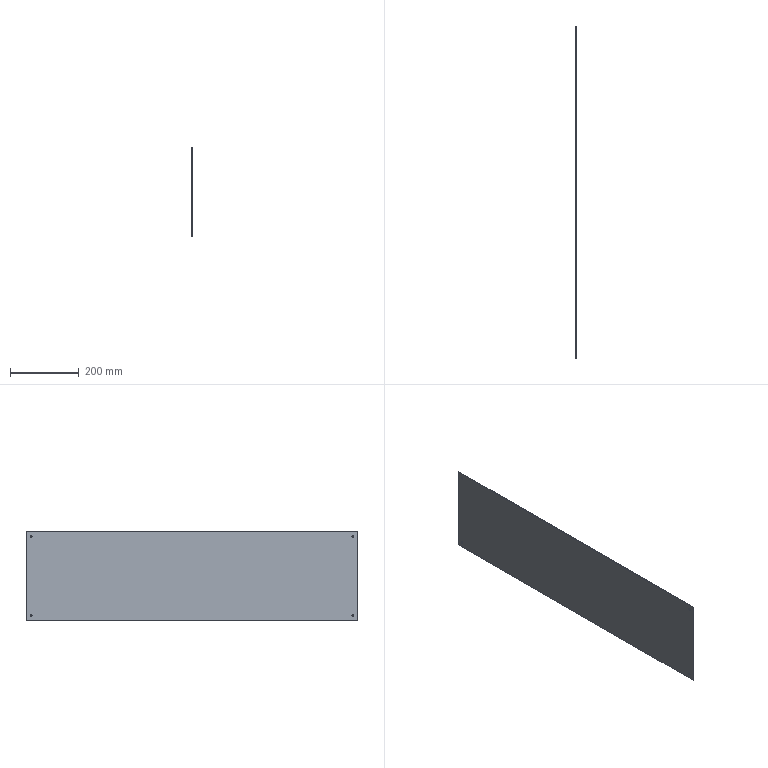Part | STEP file | PA-7-65(cover plate) | 1 solid | 14 faces | box 2 x 968 x 260 mm | volume 503203 mm3 | cylinder 8 | plane 6 | commonest cylinder face diameters 5 x8
STEP:
#1=CARTESIAN_POINT('',(0.,0.,0.));
#2=DIRECTION('',(0.,0.,1.));
#3=DIRECTION('',(1.,0.,0.));
#4=AXIS2_PLACEMENT_3D('',#1,#2,#3);
#5=CARTESIAN_POINT('',(-2.,469.,112.5));
#6=VERTEX_POINT('',#5);
#7=CARTESIAN_POINT('',(0.,469.,112.5));
#8=VERTEX_POINT('',#7);
#9=CARTESIAN_POINT('',(0.,469.,112.5));
#10=DIRECTION('',(1.,0.,0.));
#11=VECTOR('',#10,1.);
#12=LINE('',#9,#11);
#13=CARTESIAN_POINT('',(0.,469.,115.));
#14=DIRECTION('',(1.,0.,0.));
#15=DIRECTION('',(0.,0.,-1.));
#16=AXIS2_PLACEMENT_3D('',#13,#14,#15);
#17=CYLINDRICAL_SURFACE('',#16,2.5);
#18=CARTESIAN_POINT('',(6.283,0.));
#19=DIRECTION('',(0.,1.));
#20=VECTOR('',#19,1.);
#21=LINE('',#18,#20);
#22=(GEOMETRIC_REPRESENTATION_CONTEXT(2)PARAMETRIC_REPRESENTATION_CONTEXT()REPRESENTATION_CONTEXT('',''));
#23=DEFINITIONAL_REPRESENTATION('',(#21),#22);
#24=PCURVE('',#17,#23);
#25=CARTESIAN_POINT('',(0.,469.,115.));
#26=DIRECTION('',(1.,0.,0.));
#27=DIRECTION('',(0.,0.,-1.));
#28=AXIS2_PLACEMENT_3D('',#25,#26,#27);
#29=CYLINDRICAL_SURFACE('',#28,2.5);
#30=CARTESIAN_POINT('',(0.,0.));
#31=DIRECTION('',(0.,1.));
#32=VECTOR('',#31,1.);
#33=LINE('',#30,#32);
#34=(GEOMETRIC_REPRESENTATION_CONTEXT(2)PARAMETRIC_REPRESENTATION_CONTEXT()REPRESENTATION_CONTEXT('',''));
#35=DEFINITIONAL_REPRESENTATION('',(#33),#34);
#36=PCURVE('',#29,#35);
#37=SURFACE_CURVE('',#12,(#24,#36),.PCURVE_S1.);
#38=EDGE_CURVE('',#6,#8,#37,.T.);
#39=ORIENTED_EDGE('',*,*,#38,.T.);
#40=CARTESIAN_POINT('',(0.,469.,117.5));
#41=VERTEX_POINT('',#40);
#42=CARTESIAN_POINT('',(0.,469.,115.));
#43=DIRECTION('',(1.,0.,0.));
#44=DIRECTION('',(0.,0.,-1.));
#45=AXIS2_PLACEMENT_3D('',#42,#43,#44);
#46=CIRCLE('',#45,2.5);
#47=CARTESIAN_POINT('',(0.,0.));
#48=DIRECTION('',(1.,0.));
#49=VECTOR('',#48,1.);
#50=LINE('',#47,#49);
#51=(GEOMETRIC_REPRESENTATION_CONTEXT(2)PARAMETRIC_REPRESENTATION_CONTEXT()REPRESENTATION_CONTEXT('',''));
#52=DEFINITIONAL_REPRESENTATION('',(#50),#51);
#53=PCURVE('',#17,#52);
#54=CARTESIAN_POINT('',(0.,0.,0.));
#55=DIRECTION('',(1.,0.,0.));
#56=DIRECTION('',(0.,0.,-1.));
#57=AXIS2_PLACEMENT_3D('',#54,#55,#56);
#58=PLANE('',#57);
#59=CARTESIAN_POINT('',(-115.,469.));
#60=DIRECTION('',(1.,0.));
#61=AXIS2_PLACEMENT_2D('',#59,#60);
#62=CIRCLE('',#61,2.5);
#63=(GEOMETRIC_REPRESENTATION_CONTEXT(2)PARAMETRIC_REPRESENTATION_CONTEXT()REPRESENTATION_CONTEXT('',''));
#64=DEFINITIONAL_REPRESENTATION('',(#62),#63);
#65=PCURVE('',#58,#64);
#66=SURFACE_CURVE('',#46,(#53,#65),.PCURVE_S1.);
#67=EDGE_CURVE('',#41,#8,#66,.T.);
#68=ORIENTED_EDGE('',*,*,#67,.F.);
#69=CARTESIAN_POINT('',(-2.,469.,117.5));
#70=VERTEX_POINT('',#69);
#71=CARTESIAN_POINT('',(0.,469.,117.5));
#72=DIRECTION('',(1.,0.,0.));
#73=VECTOR('',#72,1.);
#74=LINE('',#71,#73);
#75=CARTESIAN_POINT('',(3.142,0.));
#76=DIRECTION('',(0.,1.));
#77=VECTOR('',#76,1.);
#78=LINE('',#75,#77);
#79=(GEOMETRIC_REPRESENTATION_CONTEXT(2)PARAMETRIC_REPRESENTATION_CONTEXT()REPRESENTATION_CONTEXT('',''));
#80=DEFINITIONAL_REPRESENTATION('',(#78),#79);
#81=PCURVE('',#17,#80);
#82=CARTESIAN_POINT('',(3.142,0.));
#83=DIRECTION('',(0.,1.));
#84=VECTOR('',#83,1.);
#85=LINE('',#82,#84);
#86=(GEOMETRIC_REPRESENTATION_CONTEXT(2)PARAMETRIC_REPRESENTATION_CONTEXT()REPRESENTATION_CONTEXT('',''));
#87=DEFINITIONAL_REPRESENTATION('',(#85),#86);
#88=PCURVE('',#29,#87);
#89=SURFACE_CURVE('',#74,(#81,#88),.PCURVE_S1.);
#90=EDGE_CURVE('',#70,#41,#89,.T.);
#91=ORIENTED_EDGE('',*,*,#90,.F.);
#92=CARTESIAN_POINT('',(-2.,469.,115.));
#93=DIRECTION('',(1.,0.,0.));
#94=DIRECTION('',(0.,0.,-1.));
#95=AXIS2_PLACEMENT_3D('',#92,#93,#94);
#96=CIRCLE('',#95,2.5);
#97=CARTESIAN_POINT('',(0.,-2.));
#98=DIRECTION('',(1.,0.));
#99=VECTOR('',#98,1.);
#100=LINE('',#97,#99);
#101=(GEOMETRIC_REPRESENTATION_CONTEXT(2)PARAMETRIC_REPRESENTATION_CONTEXT()REPRESENTATION_CONTEXT('',''));
#102=DEFINITIONAL_REPRESENTATION('',(#100),#101);
#103=PCURVE('',#17,#102);
#104=CARTESIAN_POINT('',(-2.,0.,0.));
#105=DIRECTION('',(1.,0.,0.));
#106=DIRECTION('',(0.,0.,-1.));
#107=AXIS2_PLACEMENT_3D('',#104,#105,#106);
#108=PLANE('',#107);
#109=CARTESIAN_POINT('',(-115.,469.));
#110=DIRECTION('',(1.,0.));
#111=AXIS2_PLACEMENT_2D('',#109,#110);
#112=CIRCLE('',#111,2.5);
#113=(GEOMETRIC_REPRESENTATION_CONTEXT(2)PARAMETRIC_REPRESENTATION_CONTEXT()REPRESENTATION_CONTEXT('',''));
#114=DEFINITIONAL_REPRESENTATION('',(#112),#113);
#115=PCURVE('',#108,#114);
#116=SURFACE_CURVE('',#96,(#103,#115),.PCURVE_S1.);
#117=EDGE_CURVE('',#70,#6,#116,.T.);
#118=ORIENTED_EDGE('',*,*,#117,.T.);
#119=EDGE_LOOP('',(#39,#68,#91,#118));
#120=FACE_BOUND('',#119,.F.);
#121=ADVANCED_FACE('',(#120),#17,.F.);
#122=CARTESIAN_POINT('',(-2.,-469.,112.5));
#123=VERTEX_POINT('',#122);
#124=CARTESIAN_POINT('',(0.,-469.,112.5));
#125=VERTEX_POINT('',#124);
#126=CARTESIAN_POINT('',(0.,-469.,112.5));
#127=DIRECTION('',(1.,0.,0.));
#128=VECTOR('',#127,1.);
#129=LINE('',#126,#128);
#130=CARTESIAN_POINT('',(0.,-469.,115.));
#131=DIRECTION('',(1.,0.,0.));
#132=DIRECTION('',(0.,0.,-1.));
#133=AXIS2_PLACEMENT_3D('',#130,#131,#132);
#134=CYLINDRICAL_SURFACE('',#133,2.5);
#135=CARTESIAN_POINT('',(6.283,0.));
#136=DIRECTION('',(0.,1.));
#137=VECTOR('',#136,1.);
#138=LINE('',#135,#137);
#139=(GEOMETRIC_REPRESENTATION_CONTEXT(2)PARAMETRIC_REPRESENTATION_CONTEXT()REPRESENTATION_CONTEXT('',''));
#140=DEFINITIONAL_REPRESENTATION('',(#138),#139);
#141=PCURVE('',#134,#140);
#142=CARTESIAN_POINT('',(0.,-469.,115.));
#143=DIRECTION('',(1.,0.,0.));
#144=DIRECTION('',(0.,0.,-1.));
#145=AXIS2_PLACEMENT_3D('',#142,#143,#144);
#146=CYLINDRICAL_SURFACE('',#145,2.5);
#147=CARTESIAN_POINT('',(0.,0.));
#148=DIRECTION('',(0.,1.));
#149=VECTOR('',#148,1.);
#150=LINE('',#147,#149);
#151=(GEOMETRIC_REPRESENTATION_CONTEXT(2)PARAMETRIC_REPRESENTATION_CONTEXT()REPRESENTATION_CONTEXT('',''));
#152=DEFINITIONAL_REPRESENTATION('',(#150),#151);
#153=PCURVE('',#146,#152);
#154=SURFACE_CURVE('',#129,(#141,#153),.PCURVE_S1.);
#155=EDGE_CURVE('',#123,#125,#154,.T.);
#156=ORIENTED_EDGE('',*,*,#155,.T.);
#157=CARTESIAN_POINT('',(0.,-469.,117.5));
#158=VERTEX_POINT('',#157);
#159=CARTESIAN_POINT('',(0.,-469.,115.));
#160=DIRECTION('',(1.,0.,0.));
#161=DIRECTION('',(0.,0.,-1.));
#162=AXIS2_PLACEMENT_3D('',#159,#160,#161);
#163=CIRCLE('',#162,2.5);
#164=CARTESIAN_POINT('',(0.,0.));
#165=DIRECTION('',(1.,0.));
#166=VECTOR('',#165,1.);
#167=LINE('',#164,#166);
#168=(GEOMETRIC_REPRESENTATION_CONTEXT(2)PARAMETRIC_REPRESENTATION_CONTEXT()REPRESENTATION_CONTEXT('',''));
#169=DEFINITIONAL_REPRESENTATION('',(#167),#168);
#170=PCURVE('',#134,#169);
#171=CARTESIAN_POINT('',(-115.,-469.));
#172=DIRECTION('',(1.,0.));
#173=AXIS2_PLACEMENT_2D('',#171,#172);
#174=CIRCLE('',#173,2.5);
#175=(GEOMETRIC_REPRESENTATION_CONTEXT(2)PARAMETRIC_REPRESENTATION_CONTEXT()REPRESENTATION_CONTEXT('',''));
#176=DEFINITIONAL_REPRESENTATION('',(#174),#175);
#177=PCURVE('',#58,#176);
#178=SURFACE_CURVE('',#163,(#170,#177),.PCURVE_S1.);
#179=EDGE_CURVE('',#158,#125,#178,.T.);
#180=ORIENTED_EDGE('',*,*,#179,.F.);
#181=CARTESIAN_POINT('',(-2.,-469.,117.5));
#182=VERTEX_POINT('',#181);
#183=CARTESIAN_POINT('',(0.,-469.,117.5));
#184=DIRECTION('',(1.,0.,0.));
#185=VECTOR('',#184,1.);
#186=LINE('',#183,#185);
#187=CARTESIAN_POINT('',(3.142,0.));
#188=DIRECTION('',(0.,1.));
#189=VECTOR('',#188,1.);
#190=LINE('',#187,#189);
#191=(GEOMETRIC_REPRESENTATION_CONTEXT(2)PARAMETRIC_REPRESENTATION_CONTEXT()REPRESENTATION_CONTEXT('',''));
#192=DEFINITIONAL_REPRESENTATION('',(#190),#191);
#193=PCURVE('',#134,#192);
#194=CARTESIAN_POINT('',(3.142,0.));
#195=DIRECTION('',(0.,1.));
#196=VECTOR('',#195,1.);
#197=LINE('',#194,#196);
#198=(GEOMETRIC_REPRESENTATION_CONTEXT(2)PARAMETRIC_REPRESENTATION_CONTEXT()REPRESENTATION_CONTEXT('',''));
#199=DEFINITIONAL_REPRESENTATION('',(#197),#198);
#200=PCURVE('',#146,#199);
#201=SURFACE_CURVE('',#186,(#193,#200),.PCURVE_S1.);
#202=EDGE_CURVE('',#182,#158,#201,.T.);
#203=ORIENTED_EDGE('',*,*,#202,.F.);
#204=CARTESIAN_POINT('',(-2.,-469.,115.));
#205=DIRECTION('',(1.,0.,0.));
#206=DIRECTION('',(0.,0.,-1.));
#207=AXIS2_PLACEMENT_3D('',#204,#205,#206);
#208=CIRCLE('',#207,2.5);
#209=CARTESIAN_POINT('',(0.,-2.));
#210=DIRECTION('',(1.,0.));
#211=VECTOR('',#210,1.);
#212=LINE('',#209,#211);
#213=(GEOMETRIC_REPRESENTATION_CONTEXT(2)PARAMETRIC_REPRESENTATION_CONTEXT()REPRESENTATION_CONTEXT('',''));
#214=DEFINITIONAL_REPRESENTATION('',(#212),#213);
#215=PCURVE('',#134,#214);
#216=CARTESIAN_POINT('',(-115.,-469.));
#217=DIRECTION('',(1.,0.));
#218=AXIS2_PLACEMENT_2D('',#216,#217);
#219=CIRCLE('',#218,2.5);
#220=(GEOMETRIC_REPRESENTATION_CONTEXT(2)PARAMETRIC_REPRESENTATION_CONTEXT()REPRESENTATION_CONTEXT('',''));
#221=DEFINITIONAL_REPRESENTATION('',(#219),#220);
#222=PCURVE('',#108,#221);
#223=SURFACE_CURVE('',#208,(#215,#222),.PCURVE_S1.);
#224=EDGE_CURVE('',#182,#123,#223,.T.);
#225=ORIENTED_EDGE('',*,*,#224,.T.);
#226=EDGE_LOOP('',(#156,#180,#203,#225));
#227=FACE_BOUND('',#226,.F.);
#228=ADVANCED_FACE('',(#227),#134,.F.);
#229=CARTESIAN_POINT('',(-2.,-469.,-117.5));
#230=VERTEX_POINT('',#229);
#231=CARTESIAN_POINT('',(0.,-469.,-117.5));
#232=VERTEX_POINT('',#231);
#233=CARTESIAN_POINT('',(0.,-469.,-117.5));
#234=DIRECTION('',(1.,0.,0.));
#235=VECTOR('',#234,1.);
#236=LINE('',#233,#235);
#237=CARTESIAN_POINT('',(0.,-469.,-115.));
#238=DIRECTION('',(1.,0.,0.));
#239=DIRECTION('',(0.,0.,-1.));
#240=AXIS2_PLACEMENT_3D('',#237,#238,#239);
#241=CYLINDRICAL_SURFACE('',#240,2.5);
#242=CARTESIAN_POINT('',(6.283,0.));
#243=DIRECTION('',(0.,1.));
#244=VECTOR('',#243,1.);
#245=LINE('',#242,#244);
#246=(GEOMETRIC_REPRESENTATION_CONTEXT(2)PARAMETRIC_REPRESENTATION_CONTEXT()REPRESENTATION_CONTEXT('',''));
#247=DEFINITIONAL_REPRESENTATION('',(#245),#246);
#248=PCURVE('',#241,#247);
#249=CARTESIAN_POINT('',(0.,-469.,-115.));
#250=DIRECTION('',(1.,0.,0.));
#251=DIRECTION('',(0.,0.,-1.));
#252=AXIS2_PLACEMENT_3D('',#249,#250,#251);
#253=CYLINDRICAL_SURFACE('',#252,2.5);
#254=CARTESIAN_POINT('',(0.,0.));
#255=DIRECTION('',(0.,1.));
#256=VECTOR('',#255,1.);
#257=LINE('',#254,#256);
#258=(GEOMETRIC_REPRESENTATION_CONTEXT(2)PARAMETRIC_REPRESENTATION_CONTEXT()REPRESENTATION_CONTEXT('',''));
#259=DEFINITIONAL_REPRESENTATION('',(#257),#258);
#260=PCURVE('',#253,#259);
#261=SURFACE_CURVE('',#236,(#248,#260),.PCURVE_S1.);
#262=EDGE_CURVE('',#230,#232,#261,.T.);
#263=ORIENTED_EDGE('',*,*,#262,.T.);
#264=CARTESIAN_POINT('',(0.,-469.,-112.5));
#265=VERTEX_POINT('',#264);
#266=CARTESIAN_POINT('',(0.,-469.,-115.));
#267=DIRECTION('',(1.,0.,0.));
#268=DIRECTION('',(0.,0.,-1.));
#269=AXIS2_PLACEMENT_3D('',#266,#267,#268);
#270=CIRCLE('',#269,2.5);
#271=CARTESIAN_POINT('',(0.,0.));
#272=DIRECTION('',(1.,0.));
#273=VECTOR('',#272,1.);
#274=LINE('',#271,#273);
#275=(GEOMETRIC_REPRESENTATION_CONTEXT(2)PARAMETRIC_REPRESENTATION_CONTEXT()REPRESENTATION_CONTEXT('',''));
#276=DEFINITIONAL_REPRESENTATION('',(#274),#275);
#277=PCURVE('',#241,#276);
#278=CARTESIAN_POINT('',(115.,-469.));
#279=DIRECTION('',(1.,0.));
#280=AXIS2_PLACEMENT_2D('',#278,#279);
#281=CIRCLE('',#280,2.5);
#282=(GEOMETRIC_REPRESENTATION_CONTEXT(2)PARAMETRIC_REPRESENTATION_CONTEXT()REPRESENTATION_CONTEXT('',''));
#283=DEFINITIONAL_REPRESENTATION('',(#281),#282);
#284=PCURVE('',#58,#283);
#285=SURFACE_CURVE('',#270,(#277,#284),.PCURVE_S1.);
#286=EDGE_CURVE('',#265,#232,#285,.T.);
#287=ORIENTED_EDGE('',*,*,#286,.F.);
#288=CARTESIAN_POINT('',(-2.,-469.,-112.5));
#289=VERTEX_POINT('',#288);
#290=CARTESIAN_POINT('',(0.,-469.,-112.5));
#291=DIRECTION('',(1.,0.,0.));
#292=VECTOR('',#291,1.);
#293=LINE('',#290,#292);
#294=CARTESIAN_POINT('',(3.142,0.));
#295=DIRECTION('',(0.,1.));
#296=VECTOR('',#295,1.);
#297=LINE('',#294,#296);
#298=(GEOMETRIC_REPRESENTATION_CONTEXT(2)PARAMETRIC_REPRESENTATION_CONTEXT()REPRESENTATION_CONTEXT('',''));
#299=DEFINITIONAL_REPRESENTATION('',(#297),#298);
#300=PCURVE('',#241,#299);
#301=CARTESIAN_POINT('',(3.142,0.));
#302=DIRECTION('',(0.,1.));
#303=VECTOR('',#302,1.);
#304=LINE('',#301,#303);
#305=(GEOMETRIC_REPRESENTATION_CONTEXT(2)PARAMETRIC_REPRESENTATION_CONTEXT()REPRESENTATION_CONTEXT('',''));
#306=DEFINITIONAL_REPRESENTATION('',(#304),#305);
#307=PCURVE('',#253,#306);
#308=SURFACE_CURVE('',#293,(#300,#307),.PCURVE_S1.);
#309=EDGE_CURVE('',#289,#265,#308,.T.);
#310=ORIENTED_EDGE('',*,*,#309,.F.);
#311=CARTESIAN_POINT('',(-2.,-469.,-115.));
#312=DIRECTION('',(1.,0.,0.));
#313=DIRECTION('',(0.,0.,-1.));
#314=AXIS2_PLACEMENT_3D('',#311,#312,#313);
#315=CIRCLE('',#314,2.5);
#316=CARTESIAN_POINT('',(0.,-2.));
#317=DIRECTION('',(1.,0.));
#318=VECTOR('',#317,1.);
#319=LINE('',#316,#318);
#320=(GEOMETRIC_REPRESENTATION_CONTEXT(2)PARAMETRIC_REPRESENTATION_CONTEXT()REPRESENTATION_CONTEXT('',''));
#321=DEFINITIONAL_REPRESENTATION('',(#319),#320);
#322=PCURVE('',#241,#321);
#323=CARTESIAN_POINT('',(115.,-469.));
#324=DIRECTION('',(1.,0.));
#325=AXIS2_PLACEMENT_2D('',#323,#324);
#326=CIRCLE('',#325,2.5);
#327=(GEOMETRIC_REPRESENTATION_CONTEXT(2)PARAMETRIC_REPRESENTATION_CONTEXT()REPRESENTATION_CONTEXT('',''));
#328=DEFINITIONAL_REPRESENTATION('',(#326),#327);
#329=PCURVE('',#108,#328);
#330=SURFACE_CURVE('',#315,(#322,#329),.PCURVE_S1.);
#331=EDGE_CURVE('',#289,#230,#330,.T.);
#332=ORIENTED_EDGE('',*,*,#331,.T.);
#333=EDGE_LOOP('',(#263,#287,#310,#332));
#334=FACE_BOUND('',#333,.F.);
#335=ADVANCED_FACE('',(#334),#241,.F.);
#336=CARTESIAN_POINT('',(-2.,469.,-117.5));
#337=VERTEX_POINT('',#336);
#338=CARTESIAN_POINT('',(0.,469.,-117.5));
#339=VERTEX_POINT('',#338);
#340=CARTESIAN_POINT('',(0.,469.,-117.5));
#341=DIRECTION('',(1.,0.,0.));
#342=VECTOR('',#341,1.);
#343=LINE('',#340,#342);
#344=CARTESIAN_POINT('',(0.,469.,-115.));
#345=DIRECTION('',(1.,0.,0.));
#346=DIRECTION('',(0.,0.,-1.));
#347=AXIS2_PLACEMENT_3D('',#344,#345,#346);
#348=CYLINDRICAL_SURFACE('',#347,2.5);
#349=CARTESIAN_POINT('',(6.283,0.));
#350=DIRECTION('',(0.,1.));
#351=VECTOR('',#350,1.);
#352=LINE('',#349,#351);
#353=(GEOMETRIC_REPRESENTATION_CONTEXT(2)PARAMETRIC_REPRESENTATION_CONTEXT()REPRESENTATION_CONTEXT('',''));
#354=DEFINITIONAL_REPRESENTATION('',(#352),#353);
#355=PCURVE('',#348,#354);
#356=CARTESIAN_POINT('',(0.,469.,-115.));
#357=DIRECTION('',(1.,0.,0.));
#358=DIRECTION('',(0.,0.,-1.));
#359=AXIS2_PLACEMENT_3D('',#356,#357,#358);
#360=CYLINDRICAL_SURFACE('',#359,2.5);
#361=CARTESIAN_POINT('',(0.,0.));
#362=DIRECTION('',(0.,1.));
#363=VECTOR('',#362,1.);
#364=LINE('',#361,#363);
#365=(GEOMETRIC_REPRESENTATION_CONTEXT(2)PARAMETRIC_REPRESENTATION_CONTEXT()REPRESENTATION_CONTEXT('',''));
#366=DEFINITIONAL_REPRESENTATION('',(#364),#365);
#367=PCURVE('',#360,#366);
#368=SURFACE_CURVE('',#343,(#355,#367),.PCURVE_S1.);
#369=EDGE_CURVE('',#337,#339,#368,.T.);
#370=ORIENTED_EDGE('',*,*,#369,.T.);
#371=CARTESIAN_POINT('',(0.,469.,-112.5));
#372=VERTEX_POINT('',#371);
#373=CARTESIAN_POINT('',(0.,469.,-115.));
#374=DIRECTION('',(1.,0.,0.));
#375=DIRECTION('',(0.,0.,-1.));
#376=AXIS2_PLACEMENT_3D('',#373,#374,#375);
#377=CIRCLE('',#376,2.5);
#378=CARTESIAN_POINT('',(0.,0.));
#379=DIRECTION('',(1.,0.));
#380=VECTOR('',#379,1.);
#381=LINE('',#378,#380);
#382=(GEOMETRIC_REPRESENTATION_CONTEXT(2)PARAMETRIC_REPRESENTATION_CONTEXT()REPRESENTATION_CONTEXT('',''));
#383=DEFINITIONAL_REPRESENTATION('',(#381),#382);
#384=PCURVE('',#348,#383);
#385=CARTESIAN_POINT('',(115.,469.));
#386=DIRECTION('',(1.,0.));
#387=AXIS2_PLACEMENT_2D('',#385,#386);
#388=CIRCLE('',#387,2.5);
#389=(GEOMETRIC_REPRESENTATION_CONTEXT(2)PARAMETRIC_REPRESENTATION_CONTEXT()REPRESENTATION_CONTEXT('',''));
#390=DEFINITIONAL_REPRESENTATION('',(#388),#389);
#391=PCURVE('',#58,#390);
#392=SURFACE_CURVE('',#377,(#384,#391),.PCURVE_S1.);
#393=EDGE_CURVE('',#372,#339,#392,.T.);
#394=ORIENTED_EDGE('',*,*,#393,.F.);
#395=CARTESIAN_POINT('',(-2.,469.,-112.5));
#396=VERTEX_POINT('',#395);
#397=CARTESIAN_POINT('',(0.,469.,-112.5));
#398=DIRECTION('',(1.,0.,0.));
#399=VECTOR('',#398,1.);
#400=LINE('',#397,#399);
#401=CARTESIAN_POINT('',(3.142,0.));
#402=DIRECTION('',(0.,1.));
#403=VECTOR('',#402,1.);
#404=LINE('',#401,#403);
#405=(GEOMETRIC_REPRESENTATION_CONTEXT(2)PARAMETRIC_REPRESENTATION_CONTEXT()REPRESENTATION_CONTEXT('',''));
#406=DEFINITIONAL_REPRESENTATION('',(#404),#405);
#407=PCURVE('',#348,#406);
#408=CARTESIAN_POINT('',(3.142,0.));
#409=DIRECTION('',(0.,1.));
#410=VECTOR('',#409,1.);
#411=LINE('',#408,#410);
#412=(GEOMETRIC_REPRESENTATION_CONTEXT(2)PARAMETRIC_REPRESENTATION_CONTEXT()REPRESENTATION_CONTEXT('',''));
#413=DEFINITIONAL_REPRESENTATION('',(#411),#412);
#414=PCURVE('',#360,#413);
#415=SURFACE_CURVE('',#400,(#407,#414),.PCURVE_S1.);
#416=EDGE_CURVE('',#396,#372,#415,.T.);
#417=ORIENTED_EDGE('',*,*,#416,.F.);
#418=CARTESIAN_POINT('',(-2.,469.,-115.));
#419=DIRECTION('',(1.,0.,0.));
#420=DIRECTION('',(0.,0.,-1.));
#421=AXIS2_PLACEMENT_3D('',#418,#419,#420);
#422=CIRCLE('',#421,2.5);
#423=CARTESIAN_POINT('',(0.,-2.));
#424=DIRECTION('',(1.,0.));
#425=VECTOR('',#424,1.);
#426=LINE('',#423,#425);
#427=(GEOMETRIC_REPRESENTATION_CONTEXT(2)PARAMETRIC_REPRESENTATION_CONTEXT()REPRESENTATION_CONTEXT('',''));
#428=DEFINITIONAL_REPRESENTATION('',(#426),#427);
#429=PCURVE('',#348,#428);
#430=CARTESIAN_POINT('',(115.,469.));
#431=DIRECTION('',(1.,0.));
#432=AXIS2_PLACEMENT_2D('',#430,#431);
#433=CIRCLE('',#432,2.5);
#434=(GEOMETRIC_REPRESENTATION_CONTEXT(2)PARAMETRIC_REPRESENTATION_CONTEXT()REPRESENTATION_CONTEXT('',''));
#435=DEFINITIONAL_REPRESENTATION('',(#433),#434);
#436=PCURVE('',#108,#435);
#437=SURFACE_CURVE('',#422,(#429,#436),.PCURVE_S1.);
#438=EDGE_CURVE('',#396,#337,#437,.T.);
#439=ORIENTED_EDGE('',*,*,#438,.T.);
#440=EDGE_LOOP('',(#370,#394,#417,#439));
#441=FACE_BOUND('',#440,.F.);
#442=ADVANCED_FACE('',(#441),#348,.F.);
#443=CARTESIAN_POINT('',(0.,484.,130.));
#444=VERTEX_POINT('',#443);
#445=CARTESIAN_POINT('',(0.,-484.,130.));
#446=VERTEX_POINT('',#445);
#447=CARTESIAN_POINT('',(0.,-484.,130.));
#448=DIRECTION('',(0.,-1.,0.));
#449=VECTOR('',#448,1.);
#450=LINE('',#447,#449);
#451=CARTESIAN_POINT('',(-2.,-484.,130.));
#452=DIRECTION('',(0.,0.,1.));
#453=DIRECTION('',(1.,0.,0.));
#454=AXIS2_PLACEMENT_3D('',#451,#452,#453);
#455=PLANE('',#454);
#456=CARTESIAN_POINT('',(2.,0.));
#457=DIRECTION('',(0.,-1.));
#458=VECTOR('',#457,1.);
#459=LINE('',#456,#458);
#460=(GEOMETRIC_REPRESENTATION_CONTEXT(2)PARAMETRIC_REPRESENTATION_CONTEXT()REPRESENTATION_CONTEXT('',''));
#461=DEFINITIONAL_REPRESENTATION('',(#459),#460);
#462=PCURVE('',#455,#461);
#463=CARTESIAN_POINT('',(-130.,-484.));
#464=DIRECTION('',(0.,-1.));
#465=VECTOR('',#464,1.);
#466=LINE('',#463,#465);
#467=(GEOMETRIC_REPRESENTATION_CONTEXT(2)PARAMETRIC_REPRESENTATION_CONTEXT()REPRESENTATION_CONTEXT('',''));
#468=DEFINITIONAL_REPRESENTATION('',(#466),#467);
#469=PCURVE('',#58,#468);
#470=SURFACE_CURVE('',#450,(#462,#469),.PCURVE_S1.);
#471=EDGE_CURVE('',#444,#446,#470,.T.);
#472=ORIENTED_EDGE('',*,*,#471,.F.);
#473=CARTESIAN_POINT('',(-2.,484.,130.));
#474=VERTEX_POINT('',#473);
#475=CARTESIAN_POINT('',(-2.,484.,130.));
#476=DIRECTION('',(1.,0.,0.));
#477=VECTOR('',#476,1.);
#478=LINE('',#475,#477);
#479=CARTESIAN_POINT('',(0.,968.));
#480=DIRECTION('',(1.,0.));
#481=VECTOR('',#480,1.);
#482=LINE('',#479,#481);
#483=(GEOMETRIC_REPRESENTATION_CONTEXT(2)PARAMETRIC_REPRESENTATION_CONTEXT()REPRESENTATION_CONTEXT('',''));
#484=DEFINITIONAL_REPRESENTATION('',(#482),#483);
#485=PCURVE('',#455,#484);
#486=CARTESIAN_POINT('',(-2.,484.,-130.));
#487=DIRECTION('',(0.,1.,0.));
#488=DIRECTION('',(0.,0.,1.));
#489=AXIS2_PLACEMENT_3D('',#486,#487,#488);
#490=PLANE('',#489);
#491=CARTESIAN_POINT('',(260.,0.));
#492=DIRECTION('',(0.,1.));
#493=VECTOR('',#492,1.);
#494=LINE('',#491,#493);
#495=(GEOMETRIC_REPRESENTATION_CONTEXT(2)PARAMETRIC_REPRESENTATION_CONTEXT()REPRESENTATION_CONTEXT('',''));
#496=DEFINITIONAL_REPRESENTATION('',(#494),#495);
#497=PCURVE('',#490,#496);
#498=SURFACE_CURVE('',#478,(#485,#497),.PCURVE_S1.);
#499=EDGE_CURVE('',#474,#444,#498,.T.);
#500=ORIENTED_EDGE('',*,*,#499,.F.);
#501=CARTESIAN_POINT('',(-2.,-484.,130.));
#502=VERTEX_POINT('',#501);
#503=CARTESIAN_POINT('',(-2.,-484.,130.));
#504=DIRECTION('',(0.,-1.,0.));
#505=VECTOR('',#504,1.);
#506=LINE('',#503,#505);
#507=CARTESIAN_POINT('',(0.,0.));
#508=DIRECTION('',(0.,-1.));
#509=VECTOR('',#508,1.);
#510=LINE('',#507,#509);
#511=(GEOMETRIC_REPRESENTATION_CONTEXT(2)PARAMETRIC_REPRESENTATION_CONTEXT()REPRESENTATION_CONTEXT('',''));
#512=DEFINITIONAL_REPRESENTATION('',(#510),#511);
#513=PCURVE('',#455,#512);
#514=CARTESIAN_POINT('',(-130.,-484.));
#515=DIRECTION('',(0.,-1.));
#516=VECTOR('',#515,1.);
#517=LINE('',#514,#516);
#518=(GEOMETRIC_REPRESENTATION_CONTEXT(2)PARAMETRIC_REPRESENTATION_CONTEXT()REPRESENTATION_CONTEXT('',''));
#519=DEFINITIONAL_REPRESENTATION('',(#517),#518);
#520=PCURVE('',#108,#519);
#521=SURFACE_CURVE('',#506,(#513,#520),.PCURVE_S1.);
#522=EDGE_CURVE('',#474,#502,#521,.T.);
#523=ORIENTED_EDGE('',*,*,#522,.T.);
#524=CARTESIAN_POINT('',(-2.,-484.,130.));
#525=DIRECTION('',(1.,0.,0.));
#526=VECTOR('',#525,1.);
#527=LINE('',#524,#526);
#528=CARTESIAN_POINT('',(0.,0.));
#529=DIRECTION('',(1.,0.));
#530=VECTOR('',#529,1.);
#531=LINE('',#528,#530);
#532=(GEOMETRIC_REPRESENTATION_CONTEXT(2)PARAMETRIC_REPRESENTATION_CONTEXT()REPRESENTATION_CONTEXT('',''));
#533=DEFINITIONAL_REPRESENTATION('',(#531),#532);
#534=PCURVE('',#455,#533);
#535=CARTESIAN_POINT('',(-2.,-484.,-130.));
#536=DIRECTION('',(0.,-1.,0.));
#537=DIRECTION('',(0.,0.,-1.));
#538=AXIS2_PLACEMENT_3D('',#535,#536,#537);
#539=PLANE('',#538);
#540=CARTESIAN_POINT('',(-260.,0.));
#541=DIRECTION('',(0.,1.));
#542=VECTOR('',#541,1.);
#543=LINE('',#540,#542);
#544=(GEOMETRIC_REPRESENTATION_CONTEXT(2)PARAMETRIC_REPRESENTATION_CONTEXT()REPRESENTATION_CONTEXT('',''));
#545=DEFINITIONAL_REPRESENTATION('',(#543),#544);
#546=PCURVE('',#539,#545);
#547=SURFACE_CURVE('',#527,(#534,#546),.PCURVE_S1.);
#548=EDGE_CURVE('',#502,#446,#547,.T.);
#549=ORIENTED_EDGE('',*,*,#548,.T.);
#550=EDGE_LOOP('',(#472,#500,#523,#549));
#551=FACE_BOUND('',#550,.T.);
#552=ADVANCED_FACE('',(#551),#455,.T.);
#553=CARTESIAN_POINT('',(0.,484.,-130.));
#554=VERTEX_POINT('',#553);
#555=CARTESIAN_POINT('',(0.,484.,-130.));
#556=DIRECTION('',(0.,0.,1.));
#557=VECTOR('',#556,1.);
#558=LINE('',#555,#557);
#559=CARTESIAN_POINT('',(0.,2.));
#560=DIRECTION('',(1.,0.));
#561=VECTOR('',#560,1.);
#562=LINE('',#559,#561);
#563=(GEOMETRIC_REPRESENTATION_CONTEXT(2)PARAMETRIC_REPRESENTATION_CONTEXT()REPRESENTATION_CONTEXT('',''));
#564=DEFINITIONAL_REPRESENTATION('',(#562),#563);
#565=PCURVE('',#490,#564);
#566=CARTESIAN_POINT('',(130.,484.));
#567=DIRECTION('',(-1.,0.));
#568=VECTOR('',#567,1.);
#569=LINE('',#566,#568);
#570=(GEOMETRIC_REPRESENTATION_CONTEXT(2)PARAMETRIC_REPRESENTATION_CONTEXT()REPRESENTATION_CONTEXT('',''));
#571=DEFINITIONAL_REPRESENTATION('',(#569),#570);
#572=PCURVE('',#58,#571);
#573=SURFACE_CURVE('',#558,(#565,#572),.PCURVE_S1.);
#574=EDGE_CURVE('',#554,#444,#573,.T.);
#575=ORIENTED_EDGE('',*,*,#574,.F.);
#576=CARTESIAN_POINT('',(-2.,484.,-130.));
#577=VERTEX_POINT('',#576);
#578=CARTESIAN_POINT('',(-2.,484.,-130.));
#579=DIRECTION('',(1.,0.,0.));
#580=VECTOR('',#579,1.);
#581=LINE('',#578,#580);
#582=CARTESIAN_POINT('',(0.,0.));
#583=DIRECTION('',(0.,1.));
#584=VECTOR('',#583,1.);
#585=LINE('',#582,#584);
#586=(GEOMETRIC_REPRESENTATION_CONTEXT(2)PARAMETRIC_REPRESENTATION_CONTEXT()REPRESENTATION_CONTEXT('',''));
#587=DEFINITIONAL_REPRESENTATION('',(#585),#586);
#588=PCURVE('',#490,#587);
#589=CARTESIAN_POINT('',(-2.,-484.,-130.));
#590=DIRECTION('',(0.,0.,-1.));
#591=DIRECTION('',(-1.,0.,0.));
#592=AXIS2_PLACEMENT_3D('',#589,#590,#591);
#593=PLANE('',#592);
#594=CARTESIAN_POINT('',(0.,968.));
#595=DIRECTION('',(-1.,0.));
#596=VECTOR('',#595,1.);
#597=LINE('',#594,#596);
#598=(GEOMETRIC_REPRESENTATION_CONTEXT(2)PARAMETRIC_REPRESENTATION_CONTEXT()REPRESENTATION_CONTEXT('',''));
#599=DEFINITIONAL_REPRESENTATION('',(#597),#598);
#600=PCURVE('',#593,#599);
#601=SURFACE_CURVE('',#581,(#588,#600),.PCURVE_S1.);
#602=EDGE_CURVE('',#577,#554,#601,.T.);
#603=ORIENTED_EDGE('',*,*,#602,.F.);
#604=CARTESIAN_POINT('',(-2.,484.,-130.));
#605=DIRECTION('',(0.,0.,1.));
#606=VECTOR('',#605,1.);
#607=LINE('',#604,#606);
#608=CARTESIAN_POINT('',(0.,0.));
#609=DIRECTION('',(1.,0.));
#610=VECTOR('',#609,1.);
#611=LINE('',#608,#610);
#612=(GEOMETRIC_REPRESENTATION_CONTEXT(2)PARAMETRIC_REPRESENTATION_CONTEXT()REPRESENTATION_CONTEXT('',''));
#613=DEFINITIONAL_REPRESENTATION('',(#611),#612);
#614=PCURVE('',#490,#613);
#615=CARTESIAN_POINT('',(130.,484.));
#616=DIRECTION('',(-1.,0.));
#617=VECTOR('',#616,1.);
#618=LINE('',#615,#617);
#619=(GEOMETRIC_REPRESENTATION_CONTEXT(2)PARAMETRIC_REPRESENTATION_CONTEXT()REPRESENTATION_CONTEXT('',''));
#620=DEFINITIONAL_REPRESENTATION('',(#618),#619);
#621=PCURVE('',#108,#620);
#622=SURFACE_CURVE('',#607,(#614,#621),.PCURVE_S1.);
#623=EDGE_CURVE('',#577,#474,#622,.T.);
#624=ORIENTED_EDGE('',*,*,#623,.T.);
#625=ORIENTED_EDGE('',*,*,#499,.T.);
#626=EDGE_LOOP('',(#575,#603,#624,#625));
#627=FACE_BOUND('',#626,.T.);
#628=ADVANCED_FACE('',(#627),#490,.T.);
#629=CARTESIAN_POINT('',(0.,-484.,-130.));
#630=VERTEX_POINT('',#629);
#631=CARTESIAN_POINT('',(0.,-484.,-130.));
#632=DIRECTION('',(0.,1.,0.));
#633=VECTOR('',#632,1.);
#634=LINE('',#631,#633);
#635=CARTESIAN_POINT('',(-2.,0.));
#636=DIRECTION('',(0.,1.));
#637=VECTOR('',#636,1.);
#638=LINE('',#635,#637);
#639=(GEOMETRIC_REPRESENTATION_CONTEXT(2)PARAMETRIC_REPRESENTATION_CONTEXT()REPRESENTATION_CONTEXT('',''));
#640=DEFINITIONAL_REPRESENTATION('',(#638),#639);
#641=PCURVE('',#593,#640);
#642=CARTESIAN_POINT('',(130.,-484.));
#643=DIRECTION('',(0.,1.));
#644=VECTOR('',#643,1.);
#645=LINE('',#642,#644);
#646=(GEOMETRIC_REPRESENTATION_CONTEXT(2)PARAMETRIC_REPRESENTATION_CONTEXT()REPRESENTATION_CONTEXT('',''));
#647=DEFINITIONAL_REPRESENTATION('',(#645),#646);
#648=PCURVE('',#58,#647);
#649=SURFACE_CURVE('',#634,(#641,#648),.PCURVE_S1.);
#650=EDGE_CURVE('',#630,#554,#649,.T.);
#651=ORIENTED_EDGE('',*,*,#650,.F.);
#652=CARTESIAN_POINT('',(-2.,-484.,-130.));
#653=VERTEX_POINT('',#652);
#654=CARTESIAN_POINT('',(-2.,-484.,-130.));
#655=DIRECTION('',(1.,0.,0.));
#656=VECTOR('',#655,1.);
#657=LINE('',#654,#656);
#658=CARTESIAN_POINT('',(0.,0.));
#659=DIRECTION('',(-1.,0.));
#660=VECTOR('',#659,1.);
#661=LINE('',#658,#660);
#662=(GEOMETRIC_REPRESENTATION_CONTEXT(2)PARAMETRIC_REPRESENTATION_CONTEXT()REPRESENTATION_CONTEXT('',''));
#663=DEFINITIONAL_REPRESENTATION('',(#661),#662);
#664=PCURVE('',#593,#663);
#665=CARTESIAN_POINT('',(0.,0.));
#666=DIRECTION('',(0.,1.));
#667=VECTOR('',#666,1.);
#668=LINE('',#665,#667);
#669=(GEOMETRIC_REPRESENTATION_CONTEXT(2)PARAMETRIC_REPRESENTATION_CONTEXT()REPRESENTATION_CONTEXT('',''));
#670=DEFINITIONAL_REPRESENTATION('',(#668),#669);
#671=PCURVE('',#539,#670);
#672=SURFACE_CURVE('',#657,(#664,#671),.PCURVE_S1.);
#673=EDGE_CURVE('',#653,#630,#672,.T.);
#674=ORIENTED_EDGE('',*,*,#673,.F.);
#675=CARTESIAN_POINT('',(-2.,-484.,-130.));
#676=DIRECTION('',(0.,1.,0.));
#677=VECTOR('',#676,1.);
#678=LINE('',#675,#677);
#679=CARTESIAN_POINT('',(0.,0.));
#680=DIRECTION('',(0.,1.));
#681=VECTOR('',#680,1.);
#682=LINE('',#679,#681);
#683=(GEOMETRIC_REPRESENTATION_CONTEXT(2)PARAMETRIC_REPRESENTATION_CONTEXT()REPRESENTATION_CONTEXT('',''));
#684=DEFINITIONAL_REPRESENTATION('',(#682),#683);
#685=PCURVE('',#593,#684);
#686=CARTESIAN_POINT('',(130.,-484.));
#687=DIRECTION('',(0.,1.));
#688=VECTOR('',#687,1.);
#689=LINE('',#686,#688);
#690=(GEOMETRIC_REPRESENTATION_CONTEXT(2)PARAMETRIC_REPRESENTATION_CONTEXT()REPRESENTATION_CONTEXT('',''));
#691=DEFINITIONAL_REPRESENTATION('',(#689),#690);
#692=PCURVE('',#108,#691);
#693=SURFACE_CURVE('',#678,(#685,#692),.PCURVE_S1.);
#694=EDGE_CURVE('',#653,#577,#693,.T.);
#695=ORIENTED_EDGE('',*,*,#694,.T.);
#696=ORIENTED_EDGE('',*,*,#602,.T.);
#697=EDGE_LOOP('',(#651,#674,#695,#696));
#698=FACE_BOUND('',#697,.T.);
#699=ADVANCED_FACE('',(#698),#593,.T.);
#700=CARTESIAN_POINT('',(0.,-484.,-130.));
#701=DIRECTION('',(0.,0.,-1.));
#702=VECTOR('',#701,1.);
#703=LINE('',#700,#702);
#704=CARTESIAN_POINT('',(0.,2.));
#705=DIRECTION('',(1.,0.));
#706=VECTOR('',#705,1.);
#707=LINE('',#704,#706);
#708=(GEOMETRIC_REPRESENTATION_CONTEXT(2)PARAMETRIC_REPRESENTATION_CONTEXT()REPRESENTATION_CONTEXT('',''));
#709=DEFINITIONAL_REPRESENTATION('',(#707),#708);
#710=PCURVE('',#539,#709);
#711=CARTESIAN_POINT('',(130.,-484.));
#712=DIRECTION('',(1.,0.));
#713=VECTOR('',#712,1.);
#714=LINE('',#711,#713);
#715=(GEOMETRIC_REPRESENTATION_CONTEXT(2)PARAMETRIC_REPRESENTATION_CONTEXT()REPRESENTATION_CONTEXT('',''));
#716=DEFINITIONAL_REPRESENTATION('',(#714),#715);
#717=PCURVE('',#58,#716);
#718=SURFACE_CURVE('',#703,(#710,#717),.PCURVE_S1.);
#719=EDGE_CURVE('',#446,#630,#718,.T.);
#720=ORIENTED_EDGE('',*,*,#719,.F.);
#721=ORIENTED_EDGE('',*,*,#548,.F.);
#722=CARTESIAN_POINT('',(-2.,-484.,-130.));
#723=DIRECTION('',(0.,0.,-1.));
#724=VECTOR('',#723,1.);
#725=LINE('',#722,#724);
#726=CARTESIAN_POINT('',(0.,0.));
#727=DIRECTION('',(1.,0.));
#728=VECTOR('',#727,1.);
#729=LINE('',#726,#728);
#730=(GEOMETRIC_REPRESENTATION_CONTEXT(2)PARAMETRIC_REPRESENTATION_CONTEXT()REPRESENTATION_CONTEXT('',''));
#731=DEFINITIONAL_REPRESENTATION('',(#729),#730);
#732=PCURVE('',#539,#731);
#733=CARTESIAN_POINT('',(130.,-484.));
#734=DIRECTION('',(1.,0.));
#735=VECTOR('',#734,1.);
#736=LINE('',#733,#735);
#737=(GEOMETRIC_REPRESENTATION_CONTEXT(2)PARAMETRIC_REPRESENTATION_CONTEXT()REPRESENTATION_CONTEXT('',''));
#738=DEFINITIONAL_REPRESENTATION('',(#736),#737);
#739=PCURVE('',#108,#738);
#740=SURFACE_CURVE('',#725,(#732,#739),.PCURVE_S1.);
#741=EDGE_CURVE('',#502,#653,#740,.T.);
#742=ORIENTED_EDGE('',*,*,#741,.T.);
#743=ORIENTED_EDGE('',*,*,#673,.T.);
#744=EDGE_LOOP('',(#720,#721,#742,#743));
#745=FACE_BOUND('',#744,.T.);
#746=ADVANCED_FACE('',(#745),#539,.T.);
#747=CARTESIAN_POINT('',(-2.,469.,115.));
#748=DIRECTION('',(1.,0.,0.));
#749=DIRECTION('',(0.,0.,-1.));
#750=AXIS2_PLACEMENT_3D('',#747,#748,#749);
#751=CIRCLE('',#750,2.5);
#752=CARTESIAN_POINT('',(-115.,469.));
#753=DIRECTION('',(1.,0.));
#754=AXIS2_PLACEMENT_2D('',#752,#753);
#755=CIRCLE('',#754,2.5);
#756=(GEOMETRIC_REPRESENTATION_CONTEXT(2)PARAMETRIC_REPRESENTATION_CONTEXT()REPRESENTATION_CONTEXT('',''));
#757=DEFINITIONAL_REPRESENTATION('',(#755),#756);
#758=PCURVE('',#108,#757);
#759=CARTESIAN_POINT('',(0.,-2.));
#760=DIRECTION('',(1.,0.));
#761=VECTOR('',#760,1.);
#762=LINE('',#759,#761);
#763=(GEOMETRIC_REPRESENTATION_CONTEXT(2)PARAMETRIC_REPRESENTATION_CONTEXT()REPRESENTATION_CONTEXT('',''));
#764=DEFINITIONAL_REPRESENTATION('',(#762),#763);
#765=PCURVE('',#29,#764);
#766=SURFACE_CURVE('',#751,(#758,#765),.PCURVE_S1.);
#767=EDGE_CURVE('',#6,#70,#766,.T.);
#768=ORIENTED_EDGE('',*,*,#767,.T.);
#769=ORIENTED_EDGE('',*,*,#117,.T.);
#770=EDGE_LOOP('',(#768,#769));
#771=FACE_BOUND('',#770,.T.);
#772=CARTESIAN_POINT('',(-2.,-469.,115.));
#773=DIRECTION('',(1.,0.,0.));
#774=DIRECTION('',(0.,0.,-1.));
#775=AXIS2_PLACEMENT_3D('',#772,#773,#774);
#776=CIRCLE('',#775,2.5);
#777=CARTESIAN_POINT('',(-115.,-469.));
#778=DIRECTION('',(1.,0.));
#779=AXIS2_PLACEMENT_2D('',#777,#778);
#780=CIRCLE('',#779,2.5);
#781=(GEOMETRIC_REPRESENTATION_CONTEXT(2)PARAMETRIC_REPRESENTATION_CONTEXT()REPRESENTATION_CONTEXT('',''));
#782=DEFINITIONAL_REPRESENTATION('',(#780),#781);
#783=PCURVE('',#108,#782);
#784=CARTESIAN_POINT('',(0.,-2.));
#785=DIRECTION('',(1.,0.));
#786=VECTOR('',#785,1.);
#787=LINE('',#784,#786);
#788=(GEOMETRIC_REPRESENTATION_CONTEXT(2)PARAMETRIC_REPRESENTATION_CONTEXT()REPRESENTATION_CONTEXT('',''));
#789=DEFINITIONAL_REPRESENTATION('',(#787),#788);
#790=PCURVE('',#146,#789);
#791=SURFACE_CURVE('',#776,(#783,#790),.PCURVE_S1.);
#792=EDGE_CURVE('',#123,#182,#791,.T.);
#793=ORIENTED_EDGE('',*,*,#792,.T.);
#794=ORIENTED_EDGE('',*,*,#224,.T.);
#795=EDGE_LOOP('',(#793,#794));
#796=FACE_BOUND('',#795,.T.);
#797=CARTESIAN_POINT('',(-2.,-469.,-115.));
#798=DIRECTION('',(1.,0.,0.));
#799=DIRECTION('',(0.,0.,-1.));
#800=AXIS2_PLACEMENT_3D('',#797,#798,#799);
#801=CIRCLE('',#800,2.5);
#802=CARTESIAN_POINT('',(115.,-469.));
#803=DIRECTION('',(1.,0.));
#804=AXIS2_PLACEMENT_2D('',#802,#803);
#805=CIRCLE('',#804,2.5);
#806=(GEOMETRIC_REPRESENTATION_CONTEXT(2)PARAMETRIC_REPRESENTATION_CONTEXT()REPRESENTATION_CONTEXT('',''));
#807=DEFINITIONAL_REPRESENTATION('',(#805),#806);
#808=PCURVE('',#108,#807);
#809=CARTESIAN_POINT('',(0.,-2.));
#810=DIRECTION('',(1.,0.));
#811=VECTOR('',#810,1.);
#812=LINE('',#809,#811);
#813=(GEOMETRIC_REPRESENTATION_CONTEXT(2)PARAMETRIC_REPRESENTATION_CONTEXT()REPRESENTATION_CONTEXT('',''));
#814=DEFINITIONAL_REPRESENTATION('',(#812),#813);
#815=PCURVE('',#253,#814);
#816=SURFACE_CURVE('',#801,(#808,#815),.PCURVE_S1.);
#817=EDGE_CURVE('',#230,#289,#816,.T.);
#818=ORIENTED_EDGE('',*,*,#817,.T.);
#819=ORIENTED_EDGE('',*,*,#331,.T.);
#820=EDGE_LOOP('',(#818,#819));
#821=FACE_BOUND('',#820,.T.);
#822=CARTESIAN_POINT('',(-2.,469.,-115.));
#823=DIRECTION('',(1.,0.,0.));
#824=DIRECTION('',(0.,0.,-1.));
#825=AXIS2_PLACEMENT_3D('',#822,#823,#824);
#826=CIRCLE('',#825,2.5);
#827=CARTESIAN_POINT('',(115.,469.));
#828=DIRECTION('',(1.,0.));
#829=AXIS2_PLACEMENT_2D('',#827,#828);
#830=CIRCLE('',#829,2.5);
#831=(GEOMETRIC_REPRESENTATION_CONTEXT(2)PARAMETRIC_REPRESENTATION_CONTEXT()REPRESENTATION_CONTEXT('',''));
#832=DEFINITIONAL_REPRESENTATION('',(#830),#831);
#833=PCURVE('',#108,#832);
#834=CARTESIAN_POINT('',(0.,-2.));
#835=DIRECTION('',(1.,0.));
#836=VECTOR('',#835,1.);
#837=LINE('',#834,#836);
#838=(GEOMETRIC_REPRESENTATION_CONTEXT(2)PARAMETRIC_REPRESENTATION_CONTEXT()REPRESENTATION_CONTEXT('',''));
#839=DEFINITIONAL_REPRESENTATION('',(#837),#838);
#840=PCURVE('',#360,#839);
#841=SURFACE_CURVE('',#826,(#833,#840),.PCURVE_S1.);
#842=EDGE_CURVE('',#337,#396,#841,.T.);
#843=ORIENTED_EDGE('',*,*,#842,.T.);
#844=ORIENTED_EDGE('',*,*,#438,.T.);
#845=EDGE_LOOP('',(#843,#844));
#846=FACE_BOUND('',#845,.T.);
#847=ORIENTED_EDGE('',*,*,#522,.F.);
#848=ORIENTED_EDGE('',*,*,#623,.F.);
#849=ORIENTED_EDGE('',*,*,#694,.F.);
#850=ORIENTED_EDGE('',*,*,#741,.F.);
#851=EDGE_LOOP('',(#847,#848,#849,#850));
#852=FACE_BOUND('',#851,.T.);
#853=ADVANCED_FACE('',(#771,#796,#821,#846,#852),#108,.F.);
#854=CARTESIAN_POINT('',(0.,469.,115.));
#855=DIRECTION('',(1.,0.,0.));
#856=DIRECTION('',(0.,0.,-1.));
#857=AXIS2_PLACEMENT_3D('',#854,#855,#856);
#858=CIRCLE('',#857,2.5);
#859=CARTESIAN_POINT('',(-115.,469.));
#860=DIRECTION('',(1.,0.));
#861=AXIS2_PLACEMENT_2D('',#859,#860);
#862=CIRCLE('',#861,2.5);
#863=(GEOMETRIC_REPRESENTATION_CONTEXT(2)PARAMETRIC_REPRESENTATION_CONTEXT()REPRESENTATION_CONTEXT('',''));
#864=DEFINITIONAL_REPRESENTATION('',(#862),#863);
#865=PCURVE('',#58,#864);
#866=CARTESIAN_POINT('',(0.,0.));
#867=DIRECTION('',(1.,0.));
#868=VECTOR('',#867,1.);
#869=LINE('',#866,#868);
#870=(GEOMETRIC_REPRESENTATION_CONTEXT(2)PARAMETRIC_REPRESENTATION_CONTEXT()REPRESENTATION_CONTEXT('',''));
#871=DEFINITIONAL_REPRESENTATION('',(#869),#870);
#872=PCURVE('',#29,#871);
#873=SURFACE_CURVE('',#858,(#865,#872),.PCURVE_S1.);
#874=EDGE_CURVE('',#8,#41,#873,.T.);
#875=ORIENTED_EDGE('',*,*,#874,.F.);
#876=ORIENTED_EDGE('',*,*,#67,.F.);
#877=EDGE_LOOP('',(#875,#876));
#878=FACE_BOUND('',#877,.T.);
#879=CARTESIAN_POINT('',(0.,-469.,115.));
#880=DIRECTION('',(1.,0.,0.));
#881=DIRECTION('',(0.,0.,-1.));
#882=AXIS2_PLACEMENT_3D('',#879,#880,#881);
#883=CIRCLE('',#882,2.5);
#884=CARTESIAN_POINT('',(-115.,-469.));
#885=DIRECTION('',(1.,0.));
#886=AXIS2_PLACEMENT_2D('',#884,#885);
#887=CIRCLE('',#886,2.5);
#888=(GEOMETRIC_REPRESENTATION_CONTEXT(2)PARAMETRIC_REPRESENTATION_CONTEXT()REPRESENTATION_CONTEXT('',''));
#889=DEFINITIONAL_REPRESENTATION('',(#887),#888);
#890=PCURVE('',#58,#889);
#891=CARTESIAN_POINT('',(0.,0.));
#892=DIRECTION('',(1.,0.));
#893=VECTOR('',#892,1.);
#894=LINE('',#891,#893);
#895=(GEOMETRIC_REPRESENTATION_CONTEXT(2)PARAMETRIC_REPRESENTATION_CONTEXT()REPRESENTATION_CONTEXT('',''));
#896=DEFINITIONAL_REPRESENTATION('',(#894),#895);
#897=PCURVE('',#146,#896);
#898=SURFACE_CURVE('',#883,(#890,#897),.PCURVE_S1.);
#899=EDGE_CURVE('',#125,#158,#898,.T.);
#900=ORIENTED_EDGE('',*,*,#899,.F.);
#901=ORIENTED_EDGE('',*,*,#179,.F.);
#902=EDGE_LOOP('',(#900,#901));
#903=FACE_BOUND('',#902,.T.);
#904=CARTESIAN_POINT('',(0.,-469.,-115.));
#905=DIRECTION('',(1.,0.,0.));
#906=DIRECTION('',(0.,0.,-1.));
#907=AXIS2_PLACEMENT_3D('',#904,#905,#906);
#908=CIRCLE('',#907,2.5);
#909=CARTESIAN_POINT('',(115.,-469.));
#910=DIRECTION('',(1.,0.));
#911=AXIS2_PLACEMENT_2D('',#909,#910);
#912=CIRCLE('',#911,2.5);
#913=(GEOMETRIC_REPRESENTATION_CONTEXT(2)PARAMETRIC_REPRESENTATION_CONTEXT()REPRESENTATION_CONTEXT('',''));
#914=DEFINITIONAL_REPRESENTATION('',(#912),#913);
#915=PCURVE('',#58,#914);
#916=CARTESIAN_POINT('',(0.,0.));
#917=DIRECTION('',(1.,0.));
#918=VECTOR('',#917,1.);
#919=LINE('',#916,#918);
#920=(GEOMETRIC_REPRESENTATION_CONTEXT(2)PARAMETRIC_REPRESENTATION_CONTEXT()REPRESENTATION_CONTEXT('',''));
#921=DEFINITIONAL_REPRESENTATION('',(#919),#920);
#922=PCURVE('',#253,#921);
#923=SURFACE_CURVE('',#908,(#915,#922),.PCURVE_S1.);
#924=EDGE_CURVE('',#232,#265,#923,.T.);
#925=ORIENTED_EDGE('',*,*,#924,.F.);
#926=ORIENTED_EDGE('',*,*,#286,.F.);
#927=EDGE_LOOP('',(#925,#926));
#928=FACE_BOUND('',#927,.T.);
#929=CARTESIAN_POINT('',(0.,469.,-115.));
#930=DIRECTION('',(1.,0.,0.));
#931=DIRECTION('',(0.,0.,-1.));
#932=AXIS2_PLACEMENT_3D('',#929,#930,#931);
#933=CIRCLE('',#932,2.5);
#934=CARTESIAN_POINT('',(115.,469.));
#935=DIRECTION('',(1.,0.));
#936=AXIS2_PLACEMENT_2D('',#934,#935);
#937=CIRCLE('',#936,2.5);
#938=(GEOMETRIC_REPRESENTATION_CONTEXT(2)PARAMETRIC_REPRESENTATION_CONTEXT()REPRESENTATION_CONTEXT('',''));
#939=DEFINITIONAL_REPRESENTATION('',(#937),#938);
#940=PCURVE('',#58,#939);
#941=CARTESIAN_POINT('',(0.,0.));
#942=DIRECTION('',(1.,0.));
#943=VECTOR('',#942,1.);
#944=LINE('',#941,#943);
#945=(GEOMETRIC_REPRESENTATION_CONTEXT(2)PARAMETRIC_REPRESENTATION_CONTEXT()REPRESENTATION_CONTEXT('',''));
#946=DEFINITIONAL_REPRESENTATION('',(#944),#945);
#947=PCURVE('',#360,#946);
#948=SURFACE_CURVE('',#933,(#940,#947),.PCURVE_S1.);
#949=EDGE_CURVE('',#339,#372,#948,.T.);
#950=ORIENTED_EDGE('',*,*,#949,.F.);
#951=ORIENTED_EDGE('',*,*,#393,.F.);
#952=EDGE_LOOP('',(#950,#951));
#953=FACE_BOUND('',#952,.T.);
#954=ORIENTED_EDGE('',*,*,#471,.T.);
#955=ORIENTED_EDGE('',*,*,#719,.T.);
#956=ORIENTED_EDGE('',*,*,#650,.T.);
#957=ORIENTED_EDGE('',*,*,#574,.T.);
#958=EDGE_LOOP('',(#954,#955,#956,#957));
#959=FACE_BOUND('',#958,.T.);
#960=ADVANCED_FACE('',(#878,#903,#928,#953,#959),#58,.T.);
#961=ORIENTED_EDGE('',*,*,#949,.F.);
#962=ORIENTED_EDGE('',*,*,#369,.F.);
#963=ORIENTED_EDGE('',*,*,#842,.T.);
#964=ORIENTED_EDGE('',*,*,#416,.T.);
#965=EDGE_LOOP('',(#961,#962,#963,#964));
#966=FACE_BOUND('',#965,.F.);
#967=ADVANCED_FACE('',(#966),#360,.F.);
#968=ORIENTED_EDGE('',*,*,#924,.F.);
#969=ORIENTED_EDGE('',*,*,#262,.F.);
#970=ORIENTED_EDGE('',*,*,#817,.T.);
#971=ORIENTED_EDGE('',*,*,#309,.T.);
#972=EDGE_LOOP('',(#968,#969,#970,#971));
#973=FACE_BOUND('',#972,.F.);
#974=ADVANCED_FACE('',(#973),#253,.F.);
#975=ORIENTED_EDGE('',*,*,#899,.F.);
#976=ORIENTED_EDGE('',*,*,#155,.F.);
#977=ORIENTED_EDGE('',*,*,#792,.T.);
#978=ORIENTED_EDGE('',*,*,#202,.T.);
#979=EDGE_LOOP('',(#975,#976,#977,#978));
#980=FACE_BOUND('',#979,.F.);
#981=ADVANCED_FACE('',(#980),#146,.F.);
#982=ORIENTED_EDGE('',*,*,#874,.F.);
#983=ORIENTED_EDGE('',*,*,#38,.F.);
#984=ORIENTED_EDGE('',*,*,#767,.T.);
#985=ORIENTED_EDGE('',*,*,#90,.T.);
#986=EDGE_LOOP('',(#982,#983,#984,#985));
#987=FACE_BOUND('',#986,.F.);
#988=ADVANCED_FACE('',(#987),#29,.F.);
#989=CLOSED_SHELL('',(#121,#228,#335,#442,#552,#628,#699,#746,#853,#960,#967,#974,#981,#988));
#990=MANIFOLD_SOLID_BREP('',#989);
#991=(LENGTH_UNIT()NAMED_UNIT(*)SI_UNIT(.MILLI.,.METRE.));
#992=UNCERTAINTY_MEASURE_WITH_UNIT(LENGTH_MEASURE(0.0000001),#991,'','');
#993=(NAMED_UNIT(*)PLANE_ANGLE_UNIT()SI_UNIT($,.RADIAN.));
#994=(NAMED_UNIT(*)SI_UNIT($,.STERADIAN.)SOLID_ANGLE_UNIT());
#995=(GEOMETRIC_REPRESENTATION_CONTEXT(3)GLOBAL_UNCERTAINTY_ASSIGNED_CONTEXT((#992))GLOBAL_UNIT_ASSIGNED_CONTEXT((#991,#993,#994))REPRESENTATION_CONTEXT('',''));
#996=ADVANCED_BREP_SHAPE_REPRESENTATION('',(#4,#990),#995);